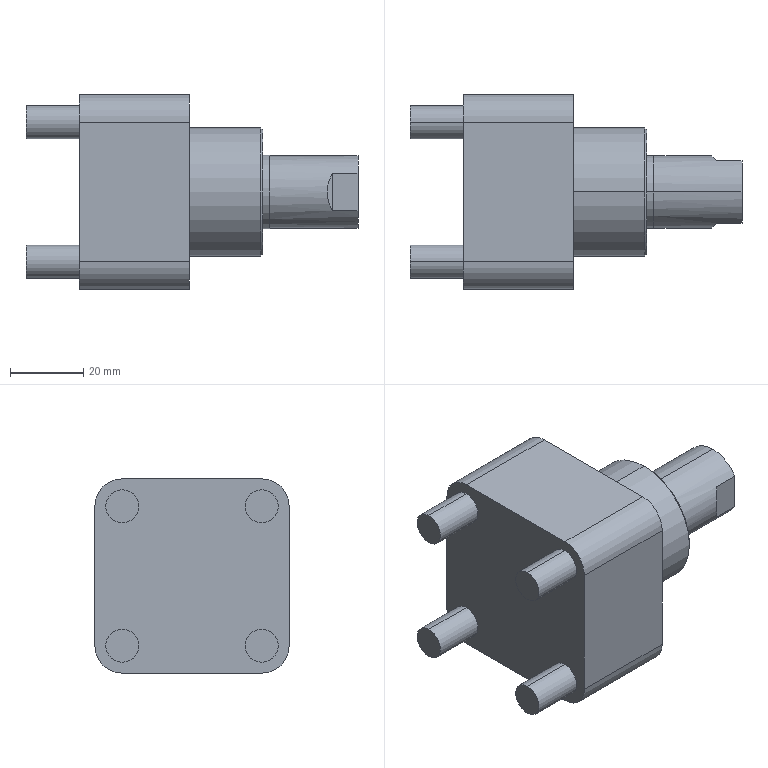Part | SolidWorks | features BaseBody 1 | 1 solid | 140 faces | box 90.5 x 53 x 53 mm | volume 107227 mm3 | plane 78 | cylinder 44 | cone 18 | commonest cylinder face diameters 9 x16 4.917 x8 11 x8 15 x4 12.5 x2 19.8 x2